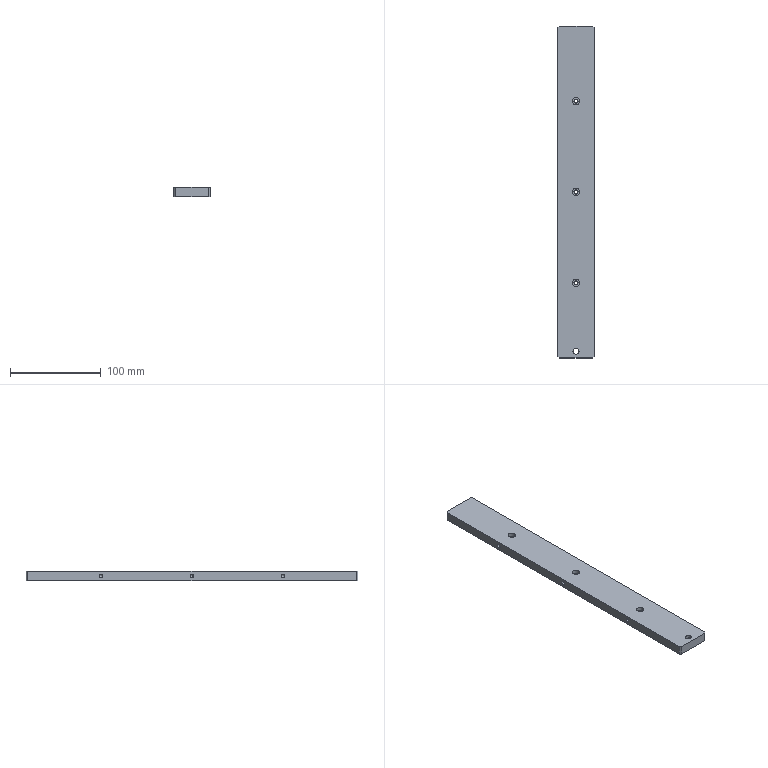Part | SolidWorks | features MirrorStock 1 | 1 solid | 50 faces | box 40 x 365 x 10 mm | volume 143435 mm3 | cylinder 26 | plane 14 | cone 10 | commonest cylinder face diameters 4.2 x6 4.5 x6 8 x6 3.3 x4 6.6 x2 11 x2
STEP:
#1=CARTESIAN_POINT('',(-4.,100.,0.4));
#2=VERTEX_POINT('',#1);
#3=CARTESIAN_POINT('',(4.,100.,0.4));
#4=VERTEX_POINT('',#3);
#5=CARTESIAN_POINT('',(0.,100.,0.4));
#6=DIRECTION('',(0.,0.,-1.));
#7=DIRECTION('',(-1.,0.,0.));
#8=AXIS2_PLACEMENT_3D('',#5,#6,#7);
#9=CIRCLE('',#8,4.);
#10=EDGE_CURVE('',#2,#4,#9,.T.);
#11=ORIENTED_EDGE('',*,*,#10,.T.);
#12=CARTESIAN_POINT('',(4.,100.,5.));
#13=VERTEX_POINT('',#12);
#14=CARTESIAN_POINT('',(4.,100.,5.));
#15=DIRECTION('',(0.,0.,1.));
#16=VECTOR('',#15,1000.);
#17=LINE('',#14,#16);
#18=EDGE_CURVE('',#4,#13,#17,.T.);
#19=ORIENTED_EDGE('',*,*,#18,.T.);
#20=CARTESIAN_POINT('',(-4.,100.,5.));
#21=VERTEX_POINT('',#20);
#22=CARTESIAN_POINT('',(0.,100.,5.));
#23=DIRECTION('',(0.,0.,-1.));
#24=DIRECTION('',(-1.,0.,0.));
#25=AXIS2_PLACEMENT_3D('',#22,#23,#24);
#26=CIRCLE('',#25,4.);
#27=EDGE_CURVE('',#21,#13,#26,.T.);
#28=ORIENTED_EDGE('',*,*,#27,.F.);
#29=CARTESIAN_POINT('',(-4.,100.,5.));
#30=DIRECTION('',(0.,0.,1.));
#31=VECTOR('',#30,1000.);
#32=LINE('',#29,#31);
#33=EDGE_CURVE('',#2,#21,#32,.T.);
#34=ORIENTED_EDGE('',*,*,#33,.F.);
#35=EDGE_LOOP('',(#11,#19,#28,#34));
#36=FACE_OUTER_BOUND('',#35,.T.);
#37=CARTESIAN_POINT('',(0.,100.,5.));
#38=DIRECTION('',(0.,0.,1.));
#39=DIRECTION('',(-1.,0.,0.));
#40=AXIS2_PLACEMENT_3D('',#37,#38,#39);
#41=CYLINDRICAL_SURFACE('',#40,4.);
#42=ADVANCED_FACE('',(#36),#41,.F.);
#43=CARTESIAN_POINT('',(-2.25,100.,-5.));
#44=VERTEX_POINT('',#43);
#45=CARTESIAN_POINT('',(2.25,100.,-5.));
#46=VERTEX_POINT('',#45);
#47=CARTESIAN_POINT('',(0.,100.,-5.));
#48=DIRECTION('',(0.,0.,-1.));
#49=DIRECTION('',(-1.,0.,0.));
#50=AXIS2_PLACEMENT_3D('',#47,#48,#49);
#51=CIRCLE('',#50,2.25);
#52=EDGE_CURVE('',#44,#46,#51,.T.);
#53=ORIENTED_EDGE('',*,*,#52,.T.);
#54=CARTESIAN_POINT('',(2.25,100.,0.4));
#55=VERTEX_POINT('',#54);
#56=CARTESIAN_POINT('',(2.25,100.,5.));
#57=DIRECTION('',(0.,0.,1.));
#58=VECTOR('',#57,1000.);
#59=LINE('',#56,#58);
#60=EDGE_CURVE('',#46,#55,#59,.T.);
#61=ORIENTED_EDGE('',*,*,#60,.T.);
#62=CARTESIAN_POINT('',(-2.25,100.,0.4));
#63=VERTEX_POINT('',#62);
#64=CARTESIAN_POINT('',(0.,100.,0.4));
#65=DIRECTION('',(0.,0.,-1.));
#66=DIRECTION('',(-1.,0.,0.));
#67=AXIS2_PLACEMENT_3D('',#64,#65,#66);
#68=CIRCLE('',#67,2.25);
#69=EDGE_CURVE('',#63,#55,#68,.T.);
#70=ORIENTED_EDGE('',*,*,#69,.F.);
#71=CARTESIAN_POINT('',(-2.25,100.,5.));
#72=DIRECTION('',(0.,0.,1.));
#73=VECTOR('',#72,1000.);
#74=LINE('',#71,#73);
#75=EDGE_CURVE('',#44,#63,#74,.T.);
#76=ORIENTED_EDGE('',*,*,#75,.F.);
#77=EDGE_LOOP('',(#53,#61,#70,#76));
#78=FACE_OUTER_BOUND('',#77,.T.);
#79=CARTESIAN_POINT('',(0.,100.,5.));
#80=DIRECTION('',(0.,0.,1.));
#81=DIRECTION('',(-1.,0.,0.));
#82=AXIS2_PLACEMENT_3D('',#79,#80,#81);
#83=CYLINDRICAL_SURFACE('',#82,2.25);
#84=ADVANCED_FACE('',(#78),#83,.F.);
#85=CARTESIAN_POINT('',(-4.,0.,0.4));
#86=VERTEX_POINT('',#85);
#87=CARTESIAN_POINT('',(4.,0.,0.4));
#88=VERTEX_POINT('',#87);
#89=CARTESIAN_POINT('',(0.,0.,0.4));
#90=DIRECTION('',(0.,0.,-1.));
#91=DIRECTION('',(-1.,0.,0.));
#92=AXIS2_PLACEMENT_3D('',#89,#90,#91);
#93=CIRCLE('',#92,4.);
#94=EDGE_CURVE('',#86,#88,#93,.T.);
#95=ORIENTED_EDGE('',*,*,#94,.T.);
#96=CARTESIAN_POINT('',(4.,0.,5.));
#97=VERTEX_POINT('',#96);
#98=CARTESIAN_POINT('',(4.,0.,5.));
#99=DIRECTION('',(0.,0.,1.));
#100=VECTOR('',#99,1000.);
#101=LINE('',#98,#100);
#102=EDGE_CURVE('',#88,#97,#101,.T.);
#103=ORIENTED_EDGE('',*,*,#102,.T.);
#104=CARTESIAN_POINT('',(-4.,0.,5.));
#105=VERTEX_POINT('',#104);
#106=CARTESIAN_POINT('',(0.,0.,5.));
#107=DIRECTION('',(0.,0.,-1.));
#108=DIRECTION('',(-1.,0.,0.));
#109=AXIS2_PLACEMENT_3D('',#106,#107,#108);
#110=CIRCLE('',#109,4.);
#111=EDGE_CURVE('',#105,#97,#110,.T.);
#112=ORIENTED_EDGE('',*,*,#111,.F.);
#113=CARTESIAN_POINT('',(-4.,0.,5.));
#114=DIRECTION('',(0.,0.,1.));
#115=VECTOR('',#114,1000.);
#116=LINE('',#113,#115);
#117=EDGE_CURVE('',#86,#105,#116,.T.);
#118=ORIENTED_EDGE('',*,*,#117,.F.);
#119=EDGE_LOOP('',(#95,#103,#112,#118));
#120=FACE_OUTER_BOUND('',#119,.T.);
#121=CARTESIAN_POINT('',(0.,0.,5.));
#122=DIRECTION('',(0.,0.,1.));
#123=DIRECTION('',(-1.,0.,0.));
#124=AXIS2_PLACEMENT_3D('',#121,#122,#123);
#125=CYLINDRICAL_SURFACE('',#124,4.);
#126=ADVANCED_FACE('',(#120),#125,.F.);
#127=CARTESIAN_POINT('',(-2.25,0.,-5.));
#128=VERTEX_POINT('',#127);
#129=CARTESIAN_POINT('',(2.25,0.,-5.));
#130=VERTEX_POINT('',#129);
#131=CARTESIAN_POINT('',(0.,0.,-5.));
#132=DIRECTION('',(0.,0.,-1.));
#133=DIRECTION('',(-1.,0.,0.));
#134=AXIS2_PLACEMENT_3D('',#131,#132,#133);
#135=CIRCLE('',#134,2.25);
#136=EDGE_CURVE('',#128,#130,#135,.T.);
#137=ORIENTED_EDGE('',*,*,#136,.T.);
#138=CARTESIAN_POINT('',(2.25,0.,0.4));
#139=VERTEX_POINT('',#138);
#140=CARTESIAN_POINT('',(2.25,0.,5.));
#141=DIRECTION('',(0.,0.,1.));
#142=VECTOR('',#141,1000.);
#143=LINE('',#140,#142);
#144=EDGE_CURVE('',#130,#139,#143,.T.);
#145=ORIENTED_EDGE('',*,*,#144,.T.);
#146=CARTESIAN_POINT('',(-2.25,0.,0.4));
#147=VERTEX_POINT('',#146);
#148=CARTESIAN_POINT('',(0.,0.,0.4));
#149=DIRECTION('',(0.,0.,-1.));
#150=DIRECTION('',(-1.,0.,0.));
#151=AXIS2_PLACEMENT_3D('',#148,#149,#150);
#152=CIRCLE('',#151,2.25);
#153=EDGE_CURVE('',#147,#139,#152,.T.);
#154=ORIENTED_EDGE('',*,*,#153,.F.);
#155=CARTESIAN_POINT('',(-2.25,0.,5.));
#156=DIRECTION('',(0.,0.,1.));
#157=VECTOR('',#156,1000.);
#158=LINE('',#155,#157);
#159=EDGE_CURVE('',#128,#147,#158,.T.);
#160=ORIENTED_EDGE('',*,*,#159,.F.);
#161=EDGE_LOOP('',(#137,#145,#154,#160));
#162=FACE_OUTER_BOUND('',#161,.T.);
#163=CARTESIAN_POINT('',(0.,0.,5.));
#164=DIRECTION('',(0.,0.,1.));
#165=DIRECTION('',(-1.,0.,0.));
#166=AXIS2_PLACEMENT_3D('',#163,#164,#165);
#167=CYLINDRICAL_SURFACE('',#166,2.25);
#168=ADVANCED_FACE('',(#162),#167,.F.);
#169=CARTESIAN_POINT('',(-4.,-100.,0.4));
#170=VERTEX_POINT('',#169);
#171=CARTESIAN_POINT('',(4.,-100.,0.4));
#172=VERTEX_POINT('',#171);
#173=CARTESIAN_POINT('',(0.,-100.,0.4));
#174=DIRECTION('',(0.,0.,-1.));
#175=DIRECTION('',(-1.,0.,0.));
#176=AXIS2_PLACEMENT_3D('',#173,#174,#175);
#177=CIRCLE('',#176,4.);
#178=EDGE_CURVE('',#170,#172,#177,.T.);
#179=ORIENTED_EDGE('',*,*,#178,.T.);
#180=CARTESIAN_POINT('',(4.,-100.,5.));
#181=VERTEX_POINT('',#180);
#182=CARTESIAN_POINT('',(4.,-100.,5.));
#183=DIRECTION('',(0.,0.,1.));
#184=VECTOR('',#183,1000.);
#185=LINE('',#182,#184);
#186=EDGE_CURVE('',#172,#181,#185,.T.);
#187=ORIENTED_EDGE('',*,*,#186,.T.);
#188=CARTESIAN_POINT('',(-4.,-100.,5.));
#189=VERTEX_POINT('',#188);
#190=CARTESIAN_POINT('',(0.,-100.,5.));
#191=DIRECTION('',(0.,0.,-1.));
#192=DIRECTION('',(-1.,0.,0.));
#193=AXIS2_PLACEMENT_3D('',#190,#191,#192);
#194=CIRCLE('',#193,4.);
#195=EDGE_CURVE('',#189,#181,#194,.T.);
#196=ORIENTED_EDGE('',*,*,#195,.F.);
#197=CARTESIAN_POINT('',(-4.,-100.,5.));
#198=DIRECTION('',(0.,0.,1.));
#199=VECTOR('',#198,1000.);
#200=LINE('',#197,#199);
#201=EDGE_CURVE('',#170,#189,#200,.T.);
#202=ORIENTED_EDGE('',*,*,#201,.F.);
#203=EDGE_LOOP('',(#179,#187,#196,#202));
#204=FACE_OUTER_BOUND('',#203,.T.);
#205=CARTESIAN_POINT('',(0.,-100.,5.));
#206=DIRECTION('',(0.,0.,1.));
#207=DIRECTION('',(-1.,0.,0.));
#208=AXIS2_PLACEMENT_3D('',#205,#206,#207);
#209=CYLINDRICAL_SURFACE('',#208,4.);
#210=ADVANCED_FACE('',(#204),#209,.F.);
#211=CARTESIAN_POINT('',(-2.25,-100.,-5.));
#212=VERTEX_POINT('',#211);
#213=CARTESIAN_POINT('',(2.25,-100.,-5.));
#214=VERTEX_POINT('',#213);
#215=CARTESIAN_POINT('',(0.,-100.,-5.));
#216=DIRECTION('',(0.,0.,-1.));
#217=DIRECTION('',(-1.,0.,0.));
#218=AXIS2_PLACEMENT_3D('',#215,#216,#217);
#219=CIRCLE('',#218,2.25);
#220=EDGE_CURVE('',#212,#214,#219,.T.);
#221=ORIENTED_EDGE('',*,*,#220,.T.);
#222=CARTESIAN_POINT('',(2.25,-100.,0.4));
#223=VERTEX_POINT('',#222);
#224=CARTESIAN_POINT('',(2.25,-100.,5.));
#225=DIRECTION('',(0.,0.,1.));
#226=VECTOR('',#225,1000.);
#227=LINE('',#224,#226);
#228=EDGE_CURVE('',#214,#223,#227,.T.);
#229=ORIENTED_EDGE('',*,*,#228,.T.);
#230=CARTESIAN_POINT('',(-2.25,-100.,0.4));
#231=VERTEX_POINT('',#230);
#232=CARTESIAN_POINT('',(0.,-100.,0.4));
#233=DIRECTION('',(0.,0.,-1.));
#234=DIRECTION('',(-1.,0.,0.));
#235=AXIS2_PLACEMENT_3D('',#232,#233,#234);
#236=CIRCLE('',#235,2.25);
#237=EDGE_CURVE('',#231,#223,#236,.T.);
#238=ORIENTED_EDGE('',*,*,#237,.F.);
#239=CARTESIAN_POINT('',(-2.25,-100.,5.));
#240=DIRECTION('',(0.,0.,1.));
#241=VECTOR('',#240,1000.);
#242=LINE('',#239,#241);
#243=EDGE_CURVE('',#212,#231,#242,.T.);
#244=ORIENTED_EDGE('',*,*,#243,.F.);
#245=EDGE_LOOP('',(#221,#229,#238,#244));
#246=FACE_OUTER_BOUND('',#245,.T.);
#247=CARTESIAN_POINT('',(0.,-100.,5.));
#248=DIRECTION('',(0.,0.,1.));
#249=DIRECTION('',(-1.,0.,0.));
#250=AXIS2_PLACEMENT_3D('',#247,#248,#249);
#251=CYLINDRICAL_SURFACE('',#250,2.25);
#252=ADVANCED_FACE('',(#246),#251,.F.);
#253=CARTESIAN_POINT('',(-6.,0.,-2.1));
#254=VERTEX_POINT('',#253);
#255=CARTESIAN_POINT('',(-6.,0.,2.1));
#256=VERTEX_POINT('',#255);
#257=CARTESIAN_POINT('',(-6.,0.,0.));
#258=DIRECTION('',(1.,0.,0.));
#259=DIRECTION('',(0.,0.,-1.));
#260=AXIS2_PLACEMENT_3D('',#257,#258,#259);
#261=CIRCLE('',#260,2.1);
#262=EDGE_CURVE('',#254,#256,#261,.T.);
#263=ORIENTED_EDGE('',*,*,#262,.T.);
#264=CARTESIAN_POINT('',(-20.,0.,2.1));
#265=VERTEX_POINT('',#264);
#266=CARTESIAN_POINT('',(-20.,0.,2.1));
#267=DIRECTION('',(-1.,0.,0.));
#268=VECTOR('',#267,1000.);
#269=LINE('',#266,#268);
#270=EDGE_CURVE('',#256,#265,#269,.T.);
#271=ORIENTED_EDGE('',*,*,#270,.T.);
#272=CARTESIAN_POINT('',(-20.,0.,-2.1));
#273=VERTEX_POINT('',#272);
#274=CARTESIAN_POINT('',(-20.,0.,0.));
#275=DIRECTION('',(1.,0.,0.));
#276=DIRECTION('',(0.,0.,-1.));
#277=AXIS2_PLACEMENT_3D('',#274,#275,#276);
#278=CIRCLE('',#277,2.1);
#279=EDGE_CURVE('',#273,#265,#278,.T.);
#280=ORIENTED_EDGE('',*,*,#279,.F.);
#281=CARTESIAN_POINT('',(-20.,0.,-2.1));
#282=DIRECTION('',(-1.,0.,0.));
#283=VECTOR('',#282,1000.);
#284=LINE('',#281,#283);
#285=EDGE_CURVE('',#254,#273,#284,.T.);
#286=ORIENTED_EDGE('',*,*,#285,.F.);
#287=EDGE_LOOP('',(#263,#271,#280,#286));
#288=FACE_OUTER_BOUND('',#287,.T.);
#289=CARTESIAN_POINT('',(-20.,0.,0.));
#290=DIRECTION('',(-1.,0.,0.));
#291=DIRECTION('',(0.,0.,-1.));
#292=AXIS2_PLACEMENT_3D('',#289,#290,#291);
#293=CYLINDRICAL_SURFACE('',#292,2.1);
#294=ADVANCED_FACE('',(#288),#293,.F.);
#295=CARTESIAN_POINT('',(-4.738,0.,0.));
#296=VERTEX_POINT('',#295);
#297=CARTESIAN_POINT('',(-6.,0.,-2.1));
#298=DIRECTION('',(-0.515,0.,-0.8572));
#299=VECTOR('',#298,1000.);
#300=LINE('',#297,#299);
#301=EDGE_CURVE('',#296,#254,#300,.T.);
#302=ORIENTED_EDGE('',*,*,#301,.F.);
#303=CARTESIAN_POINT('',(-6.,0.,2.1));
#304=DIRECTION('',(-0.515,0.,0.8572));
#305=VECTOR('',#304,1000.);
#306=LINE('',#303,#305);
#307=EDGE_CURVE('',#296,#256,#306,.T.);
#308=ORIENTED_EDGE('',*,*,#307,.T.);
#309=ORIENTED_EDGE('',*,*,#262,.F.);
#310=EDGE_LOOP('',(#302,#308,#309));
#311=FACE_OUTER_BOUND('',#310,.T.);
#312=CARTESIAN_POINT('',(-6.,0.,0.));
#313=DIRECTION('',(-1.,0.,0.));
#314=DIRECTION('',(0.,0.,-1.));
#315=AXIS2_PLACEMENT_3D('',#312,#313,#314);
#316=CONICAL_SURFACE('',#315,2.1,1.03);
#317=ADVANCED_FACE('',(#311),#316,.F.);
#318=CARTESIAN_POINT('',(-6.,100.,-2.1));
#319=VERTEX_POINT('',#318);
#320=CARTESIAN_POINT('',(-6.,100.,2.1));
#321=VERTEX_POINT('',#320);
#322=CARTESIAN_POINT('',(-6.,100.,0.));
#323=DIRECTION('',(1.,0.,0.));
#324=DIRECTION('',(0.,0.,-1.));
#325=AXIS2_PLACEMENT_3D('',#322,#323,#324);
#326=CIRCLE('',#325,2.1);
#327=EDGE_CURVE('',#319,#321,#326,.T.);
#328=ORIENTED_EDGE('',*,*,#327,.T.);
#329=CARTESIAN_POINT('',(-20.,100.,2.1));
#330=VERTEX_POINT('',#329);
#331=CARTESIAN_POINT('',(-20.,100.,2.1));
#332=DIRECTION('',(-1.,0.,0.));
#333=VECTOR('',#332,1000.);
#334=LINE('',#331,#333);
#335=EDGE_CURVE('',#321,#330,#334,.T.);
#336=ORIENTED_EDGE('',*,*,#335,.T.);
#337=CARTESIAN_POINT('',(-20.,100.,-2.1));
#338=VERTEX_POINT('',#337);
#339=CARTESIAN_POINT('',(-20.,100.,0.));
#340=DIRECTION('',(1.,0.,0.));
#341=DIRECTION('',(0.,0.,-1.));
#342=AXIS2_PLACEMENT_3D('',#339,#340,#341);
#343=CIRCLE('',#342,2.1);
#344=EDGE_CURVE('',#338,#330,#343,.T.);
#345=ORIENTED_EDGE('',*,*,#344,.F.);
#346=CARTESIAN_POINT('',(-20.,100.,-2.1));
#347=DIRECTION('',(-1.,0.,0.));
#348=VECTOR('',#347,1000.);
#349=LINE('',#346,#348);
#350=EDGE_CURVE('',#319,#338,#349,.T.);
#351=ORIENTED_EDGE('',*,*,#350,.F.);
#352=EDGE_LOOP('',(#328,#336,#345,#351));
#353=FACE_OUTER_BOUND('',#352,.T.);
#354=CARTESIAN_POINT('',(-20.,100.,0.));
#355=DIRECTION('',(-1.,0.,0.));
#356=DIRECTION('',(0.,0.,-1.));
#357=AXIS2_PLACEMENT_3D('',#354,#355,#356);
#358=CYLINDRICAL_SURFACE('',#357,2.1);
#359=ADVANCED_FACE('',(#353),#358,.F.);
#360=CARTESIAN_POINT('',(-4.738,100.,0.));
#361=VERTEX_POINT('',#360);
#362=CARTESIAN_POINT('',(-6.,100.,-2.1));
#363=DIRECTION('',(-0.515,0.,-0.8572));
#364=VECTOR('',#363,1000.);
#365=LINE('',#362,#364);
#366=EDGE_CURVE('',#361,#319,#365,.T.);
#367=ORIENTED_EDGE('',*,*,#366,.F.);
#368=CARTESIAN_POINT('',(-6.,100.,2.1));
#369=DIRECTION('',(-0.515,0.,0.8572));
#370=VECTOR('',#369,1000.);
#371=LINE('',#368,#370);
#372=EDGE_CURVE('',#361,#321,#371,.T.);
#373=ORIENTED_EDGE('',*,*,#372,.T.);
#374=ORIENTED_EDGE('',*,*,#327,.F.);
#375=EDGE_LOOP('',(#367,#373,#374));
#376=FACE_OUTER_BOUND('',#375,.T.);
#377=CARTESIAN_POINT('',(-6.,100.,0.));
#378=DIRECTION('',(-1.,0.,0.));
#379=DIRECTION('',(0.,0.,-1.));
#380=AXIS2_PLACEMENT_3D('',#377,#378,#379);
#381=CONICAL_SURFACE('',#380,2.1,1.03);
#382=ADVANCED_FACE('',(#376),#381,.F.);
#383=CARTESIAN_POINT('',(-6.,-100.,-2.1));
#384=VERTEX_POINT('',#383);
#385=CARTESIAN_POINT('',(-6.,-100.,2.1));
#386=VERTEX_POINT('',#385);
#387=CARTESIAN_POINT('',(-6.,-100.,0.));
#388=DIRECTION('',(1.,0.,0.));
#389=DIRECTION('',(0.,0.,-1.));
#390=AXIS2_PLACEMENT_3D('',#387,#388,#389);
#391=CIRCLE('',#390,2.1);
#392=EDGE_CURVE('',#384,#386,#391,.T.);
#393=ORIENTED_EDGE('',*,*,#392,.T.);
#394=CARTESIAN_POINT('',(-20.,-100.,2.1));
#395=VERTEX_POINT('',#394);
#396=CARTESIAN_POINT('',(-20.,-100.,2.1));
#397=DIRECTION('',(-1.,0.,0.));
#398=VECTOR('',#397,1000.);
#399=LINE('',#396,#398);
#400=EDGE_CURVE('',#386,#395,#399,.T.);
#401=ORIENTED_EDGE('',*,*,#400,.T.);
#402=CARTESIAN_POINT('',(-20.,-100.,-2.1));
#403=VERTEX_POINT('',#402);
#404=CARTESIAN_POINT('',(-20.,-100.,0.));
#405=DIRECTION('',(1.,0.,0.));
#406=DIRECTION('',(0.,0.,-1.));
#407=AXIS2_PLACEMENT_3D('',#404,#405,#406);
#408=CIRCLE('',#407,2.1);
#409=EDGE_CURVE('',#403,#395,#408,.T.);
#410=ORIENTED_EDGE('',*,*,#409,.F.);
#411=CARTESIAN_POINT('',(-20.,-100.,-2.1));
#412=DIRECTION('',(-1.,0.,0.));
#413=VECTOR('',#412,1000.);
#414=LINE('',#411,#413);
#415=EDGE_CURVE('',#384,#403,#414,.T.);
#416=ORIENTED_EDGE('',*,*,#415,.F.);
#417=EDGE_LOOP('',(#393,#401,#410,#416));
#418=FACE_OUTER_BOUND('',#417,.T.);
#419=CARTESIAN_POINT('',(-20.,-100.,0.));
#420=DIRECTION('',(-1.,0.,0.));
#421=DIRECTION('',(0.,0.,-1.));
#422=AXIS2_PLACEMENT_3D('',#419,#420,#421);
#423=CYLINDRICAL_SURFACE('',#422,2.1);
#424=ADVANCED_FACE('',(#418),#423,.F.);
#425=CARTESIAN_POINT('',(-4.738,-100.,0.));
#426=VERTEX_POINT('',#425);
#427=CARTESIAN_POINT('',(-6.,-100.,-2.1));
#428=DIRECTION('',(-0.515,0.,-0.8572));
#429=VECTOR('',#428,1000.);
#430=LINE('',#427,#429);
#431=EDGE_CURVE('',#426,#384,#430,.T.);
#432=ORIENTED_EDGE('',*,*,#431,.F.);
#433=CARTESIAN_POINT('',(-6.,-100.,2.1));
#434=DIRECTION('',(-0.515,0.,0.8572));
#435=VECTOR('',#434,1000.);
#436=LINE('',#433,#435);
#437=EDGE_CURVE('',#426,#386,#436,.T.);
#438=ORIENTED_EDGE('',*,*,#437,.T.);
#439=ORIENTED_EDGE('',*,*,#392,.F.);
#440=EDGE_LOOP('',(#432,#438,#439));
#441=FACE_OUTER_BOUND('',#440,.T.);
#442=CARTESIAN_POINT('',(-6.,-100.,0.));
#443=DIRECTION('',(-1.,0.,0.));
#444=DIRECTION('',(0.,0.,-1.));
#445=AXIS2_PLACEMENT_3D('',#442,#443,#444);
#446=CONICAL_SURFACE('',#445,2.1,1.03);
#447=ADVANCED_FACE('',(#441),#446,.F.);
#448=CARTESIAN_POINT('',(5.5,-175.,1.8));
#449=VERTEX_POINT('',#448);
#450=CARTESIAN_POINT('',(-5.5,-175.,1.8));
#451=VERTEX_POINT('',#450);
#452=CARTESIAN_POINT('',(0.,-175.,1.8));
#453=DIRECTION('',(0.,0.,1.));
#454=DIRECTION('',(1.,0.,0.));
#455=AXIS2_PLACEMENT_3D('',#452,#453,#454);
#456=CIRCLE('',#455,5.5);
#457=EDGE_CURVE('',#449,#451,#456,.T.);
#458=ORIENTED_EDGE('',*,*,#457,.T.);
#459=CARTESIAN_POINT('',(-5.5,-175.,-5.));
#460=VERTEX_POINT('',#459);
#461=CARTESIAN_POINT('',(-5.5,-175.,-5.));
#462=DIRECTION('',(0.,0.,-1.));
#463=VECTOR('',#462,1000.);
#464=LINE('',#461,#463);
#465=EDGE_CURVE('',#451,#460,#464,.T.);
#466=ORIENTED_EDGE('',*,*,#465,.T.);
#467=CARTESIAN_POINT('',(5.5,-175.,-5.));
#468=VERTEX_POINT('',#467);
#469=CARTESIAN_POINT('',(0.,-175.,-5.));
#470=DIRECTION('',(0.,0.,1.));
#471=DIRECTION('',(1.,0.,0.));
#472=AXIS2_PLACEMENT_3D('',#469,#470,#471);
#473=CIRCLE('',#472,5.5);
#474=EDGE_CURVE('',#468,#460,#473,.T.);
#475=ORIENTED_EDGE('',*,*,#474,.F.);
#476=CARTESIAN_POINT('',(5.5,-175.,-5.));
#477=DIRECTION('',(0.,0.,-1.));
#478=VECTOR('',#477,1000.);
#479=LINE('',#476,#478);
#480=EDGE_CURVE('',#449,#468,#479,.T.);
#481=ORIENTED_EDGE('',*,*,#480,.F.);
#482=EDGE_LOOP('',(#458,#466,#475,#481));
#483=FACE_OUTER_BOUND('',#482,.T.);
#484=CARTESIAN_POINT('',(0.,-175.,-5.));
#485=DIRECTION('',(0.,0.,-1.));
#486=DIRECTION('',(1.,0.,0.));
#487=AXIS2_PLACEMENT_3D('',#484,#485,#486);
#488=CYLINDRICAL_SURFACE('',#487,5.5);
#489=ADVANCED_FACE('',(#483),#488,.F.);
#490=CARTESIAN_POINT('',(3.3,-175.,5.));
#491=VERTEX_POINT('',#490);
#492=CARTESIAN_POINT('',(-3.3,-175.,5.));
#493=VERTEX_POINT('',#492);
#494=CARTESIAN_POINT('',(0.,-175.,5.));
#495=DIRECTION('',(0.,0.,1.));
#496=DIRECTION('',(1.,0.,0.));
#497=AXIS2_PLACEMENT_3D('',#494,#495,#496);
#498=CIRCLE('',#497,3.3);
#499=EDGE_CURVE('',#491,#493,#498,.T.);
#500=ORIENTED_EDGE('',*,*,#499,.T.);
#501=CARTESIAN_POINT('',(-3.3,-175.,1.8));
#502=VERTEX_POINT('',#501);
#503=CARTESIAN_POINT('',(-3.3,-175.,-5.));
#504=DIRECTION('',(0.,0.,-1.));
#505=VECTOR('',#504,1000.);
#506=LINE('',#503,#505);
#507=EDGE_CURVE('',#493,#502,#506,.T.);
#508=ORIENTED_EDGE('',*,*,#507,.T.);
#509=CARTESIAN_POINT('',(3.3,-175.,1.8));
#510=VERTEX_POINT('',#509);
#511=CARTESIAN_POINT('',(0.,-175.,1.8));
#512=DIRECTION('',(0.,0.,1.));
#513=DIRECTION('',(1.,0.,0.));
#514=AXIS2_PLACEMENT_3D('',#511,#512,#513);
#515=CIRCLE('',#514,3.3);
#516=EDGE_CURVE('',#510,#502,#515,.T.);
#517=ORIENTED_EDGE('',*,*,#516,.F.);
#518=CARTESIAN_POINT('',(3.3,-175.,-5.));
#519=DIRECTION('',(0.,0.,-1.));
#520=VECTOR('',#519,1000.);
#521=LINE('',#518,#520);
#522=EDGE_CURVE('',#491,#510,#521,.T.);
#523=ORIENTED_EDGE('',*,*,#522,.F.);
#524=EDGE_LOOP('',(#500,#508,#517,#523));
#525=FACE_OUTER_BOUND('',#524,.T.);
#526=CARTESIAN_POINT('',(0.,-175.,-5.));
#527=DIRECTION('',(0.,0.,-1.));
#528=DIRECTION('',(1.,0.,0.));
#529=AXIS2_PLACEMENT_3D('',#526,#527,#528);
#530=CYLINDRICAL_SURFACE('',#529,3.3);
#531=ADVANCED_FACE('',(#525),#530,.F.);
#532=CARTESIAN_POINT('',(-10.,172.4,-1.65));
#533=VERTEX_POINT('',#532);
#534=CARTESIAN_POINT('',(-10.,172.4,1.65));
#535=VERTEX_POINT('',#534);
#536=CARTESIAN_POINT('',(-10.,172.4,0.));
#537=DIRECTION('',(0.,-1.,0.));
#538=DIRECTION('',(0.,0.,-1.));
#539=AXIS2_PLACEMENT_3D('',#536,#537,#538);
#540=CIRCLE('',#539,1.65);
#541=EDGE_CURVE('',#533,#535,#540,.T.);
#542=ORIENTED_EDGE('',*,*,#541,.T.);
#543=CARTESIAN_POINT('',(-10.,182.5,1.65));
#544=VERTEX_POINT('',#543);
#545=CARTESIAN_POINT('',(-10.,182.5,1.65));
#546=DIRECTION('',(0.,1.,0.));
#547=VECTOR('',#546,1000.);
#548=LINE('',#545,#547);
#549=EDGE_CURVE('',#535,#544,#548,.T.);
#550=ORIENTED_EDGE('',*,*,#549,.T.);
#551=CARTESIAN_POINT('',(-10.,182.5,-1.65));
#552=VERTEX_POINT('',#551);
#553=CARTESIAN_POINT('',(-10.,182.5,0.));
#554=DIRECTION('',(0.,-1.,0.));
#555=DIRECTION('',(0.,0.,-1.));
#556=AXIS2_PLACEMENT_3D('',#553,#554,#555);
#557=CIRCLE('',#556,1.65);
#558=EDGE_CURVE('',#552,#544,#557,.T.);
#559=ORIENTED_EDGE('',*,*,#558,.F.);
#560=CARTESIAN_POINT('',(-10.,182.5,-1.65));
#561=DIRECTION('',(0.,1.,0.));
#562=VECTOR('',#561,1000.);
#563=LINE('',#560,#562);
#564=EDGE_CURVE('',#533,#552,#563,.T.);
#565=ORIENTED_EDGE('',*,*,#564,.F.);
#566=EDGE_LOOP('',(#542,#550,#559,#565));
#567=FACE_OUTER_BOUND('',#566,.T.);
#568=CARTESIAN_POINT('',(-10.,182.5,0.));
#569=DIRECTION('',(0.,1.,0.));
#570=DIRECTION('',(0.,0.,-1.));
#571=AXIS2_PLACEMENT_3D('',#568,#569,#570);
#572=CYLINDRICAL_SURFACE('',#571,1.65);
#573=ADVANCED_FACE('',(#567),#572,.F.);
#574=CARTESIAN_POINT('',(-10.,171.409,0.));
#575=VERTEX_POINT('',#574);
#576=CARTESIAN_POINT('',(-10.,172.4,-1.65));
#577=DIRECTION('',(0.,0.515,-0.8572));
#578=VECTOR('',#577,1000.);
#579=LINE('',#576,#578);
#580=EDGE_CURVE('',#575,#533,#579,.T.);
#581=ORIENTED_EDGE('',*,*,#580,.F.);
#582=CARTESIAN_POINT('',(-10.,172.4,1.65));
#583=DIRECTION('',(0.,0.515,0.8572));
#584=VECTOR('',#583,1000.);
#585=LINE('',#582,#584);
#586=EDGE_CURVE('',#575,#535,#585,.T.);
#587=ORIENTED_EDGE('',*,*,#586,.T.);
#588=ORIENTED_EDGE('',*,*,#541,.F.);
#589=EDGE_LOOP('',(#581,#587,#588));
#590=FACE_OUTER_BOUND('',#589,.T.);
#591=CARTESIAN_POINT('',(-10.,172.4,0.));
#592=DIRECTION('',(0.,1.,0.));
#593=DIRECTION('',(0.,0.,-1.));
#594=AXIS2_PLACEMENT_3D('',#591,#592,#593);
#595=CONICAL_SURFACE('',#594,1.65,1.03);
#596=ADVANCED_FACE('',(#590),#595,.F.);
#597=CARTESIAN_POINT('',(10.,172.4,-1.65));
#598=VERTEX_POINT('',#597);
#599=CARTESIAN_POINT('',(10.,172.4,1.65));
#600=VERTEX_POINT('',#599);
#601=CARTESIAN_POINT('',(10.,172.4,0.));
#602=DIRECTION('',(0.,-1.,0.));
#603=DIRECTION('',(0.,0.,-1.));
#604=AXIS2_PLACEMENT_3D('',#601,#602,#603);
#605=CIRCLE('',#604,1.65);
#606=EDGE_CURVE('',#598,#600,#605,.T.);
#607=ORIENTED_EDGE('',*,*,#606,.T.);
#608=CARTESIAN_POINT('',(10.,182.5,1.65));
#609=VERTEX_POINT('',#608);
#610=CARTESIAN_POINT('',(10.,182.5,1.65));
#611=DIRECTION('',(0.,1.,0.));
#612=VECTOR('',#611,1000.);
#613=LINE('',#610,#612);
#614=EDGE_CURVE('',#600,#609,#613,.T.);
#615=ORIENTED_EDGE('',*,*,#614,.T.);
#616=CARTESIAN_POINT('',(10.,182.5,-1.65));
#617=VERTEX_POINT('',#616);
#618=CARTESIAN_POINT('',(10.,182.5,0.));
#619=DIRECTION('',(0.,-1.,0.));
#620=DIRECTION('',(0.,0.,-1.));
#621=AXIS2_PLACEMENT_3D('',#618,#619,#620);
#622=CIRCLE('',#621,1.65);
#623=EDGE_CURVE('',#617,#609,#622,.T.);
#624=ORIENTED_EDGE('',*,*,#623,.F.);
#625=CARTESIAN_POINT('',(10.,182.5,-1.65));
#626=DIRECTION('',(0.,1.,0.));
#627=VECTOR('',#626,1000.);
#628=LINE('',#625,#627);
#629=EDGE_CURVE('',#598,#617,#628,.T.);
#630=ORIENTED_EDGE('',*,*,#629,.F.);
#631=EDGE_LOOP('',(#607,#615,#624,#630));
#632=FACE_OUTER_BOUND('',#631,.T.);
#633=CARTESIAN_POINT('',(10.,182.5,0.));
#634=DIRECTION('',(0.,1.,0.));
#635=DIRECTION('',(0.,0.,-1.));
#636=AXIS2_PLACEMENT_3D('',#633,#634,#635);
#637=CYLINDRICAL_SURFACE('',#636,1.65);
#638=ADVANCED_FACE('',(#632),#637,.F.);
#639=CARTESIAN_POINT('',(10.,171.409,0.));
#640=VERTEX_POINT('',#639);
#641=CARTESIAN_POINT('',(10.,172.4,-1.65));
#642=DIRECTION('',(0.,0.515,-0.8572));
#643=VECTOR('',#642,1000.);
#644=LINE('',#641,#643);
#645=EDGE_CURVE('',#640,#598,#644,.T.);
#646=ORIENTED_EDGE('',*,*,#645,.F.);
#647=CARTESIAN_POINT('',(10.,172.4,1.65));
#648=DIRECTION('',(0.,0.515,0.8572));
#649=VECTOR('',#648,1000.);
#650=LINE('',#647,#649);
#651=EDGE_CURVE('',#640,#600,#650,.T.);
#652=ORIENTED_EDGE('',*,*,#651,.T.);
#653=ORIENTED_EDGE('',*,*,#606,.F.);
#654=EDGE_LOOP('',(#646,#652,#653));
#655=FACE_OUTER_BOUND('',#654,.T.);
#656=CARTESIAN_POINT('',(10.,172.4,0.));
#657=DIRECTION('',(0.,1.,0.));
#658=DIRECTION('',(0.,0.,-1.));
#659=AXIS2_PLACEMENT_3D('',#656,#657,#658);
#660=CONICAL_SURFACE('',#659,1.65,1.03);
#661=ADVANCED_FACE('',(#655),#660,.F.);
#662=ORIENTED_EDGE('',*,*,#279,.T.);
#663=CARTESIAN_POINT('',(-20.,0.,0.));
#664=DIRECTION('',(1.,0.,0.));
#665=DIRECTION('',(0.,0.,-1.));
#666=AXIS2_PLACEMENT_3D('',#663,#664,#665);
#667=CIRCLE('',#666,2.1);
#668=EDGE_CURVE('',#265,#273,#667,.T.);
#669=ORIENTED_EDGE('',*,*,#668,.T.);
#670=EDGE_LOOP('',(#662,#669));
#671=FACE_BOUND('',#670,.T.);
#672=ORIENTED_EDGE('',*,*,#344,.T.);
#673=CARTESIAN_POINT('',(-20.,100.,0.));
#674=DIRECTION('',(1.,0.,0.));
#675=DIRECTION('',(0.,0.,-1.));
#676=AXIS2_PLACEMENT_3D('',#673,#674,#675);
#677=CIRCLE('',#676,2.1);
#678=EDGE_CURVE('',#330,#338,#677,.T.);
#679=ORIENTED_EDGE('',*,*,#678,.T.);
#680=EDGE_LOOP('',(#672,#679));
#681=FACE_BOUND('',#680,.T.);
#682=ORIENTED_EDGE('',*,*,#409,.T.);
#683=CARTESIAN_POINT('',(-20.,-100.,0.));
#684=DIRECTION('',(1.,0.,0.));
#685=DIRECTION('',(0.,0.,-1.));
#686=AXIS2_PLACEMENT_3D('',#683,#684,#685);
#687=CIRCLE('',#686,2.1);
#688=EDGE_CURVE('',#395,#403,#687,.T.);
#689=ORIENTED_EDGE('',*,*,#688,.T.);
#690=EDGE_LOOP('',(#682,#689));
#691=FACE_BOUND('',#690,.T.);
#692=CARTESIAN_POINT('',(-20.,180.5,5.));
#693=VERTEX_POINT('',#692);
#694=CARTESIAN_POINT('',(-20.,-180.5,5.));
#695=VERTEX_POINT('',#694);
#696=CARTESIAN_POINT('',(-20.,-182.5,5.));
#697=DIRECTION('',(0.,-1.,0.));
#698=VECTOR('',#697,1000.);
#699=LINE('',#696,#698);
#700=EDGE_CURVE('',#693,#695,#699,.T.);
#701=ORIENTED_EDGE('',*,*,#700,.F.);
#702=CARTESIAN_POINT('',(-20.,180.5,-5.));
#703=VERTEX_POINT('',#702);
#704=CARTESIAN_POINT('',(-20.,180.5,-5.));
#705=DIRECTION('',(0.,0.,1.));
#706=VECTOR('',#705,1000.);
#707=LINE('',#704,#706);
#708=EDGE_CURVE('',#703,#693,#707,.T.);
#709=ORIENTED_EDGE('',*,*,#708,.F.);
#710=CARTESIAN_POINT('',(-20.,-180.5,-5.));
#711=VERTEX_POINT('',#710);
#712=CARTESIAN_POINT('',(-20.,-182.5,-5.));
#713=DIRECTION('',(0.,-1.,0.));
#714=VECTOR('',#713,1000.);
#715=LINE('',#712,#714);
#716=EDGE_CURVE('',#703,#711,#715,.T.);
#717=ORIENTED_EDGE('',*,*,#716,.T.);
#718=CARTESIAN_POINT('',(-20.,-180.5,-5.));
#719=DIRECTION('',(0.,0.,-1.));
#720=VECTOR('',#719,1000.);
#721=LINE('',#718,#720);
#722=EDGE_CURVE('',#695,#711,#721,.T.);
#723=ORIENTED_EDGE('',*,*,#722,.F.);
#724=EDGE_LOOP('',(#701,#709,#717,#723));
#725=FACE_OUTER_BOUND('',#724,.T.);
#726=CARTESIAN_POINT('',(-20.,-182.5,-5.));
#727=DIRECTION('',(1.,0.,0.));
#728=DIRECTION('',(0.,0.,1.));
#729=AXIS2_PLACEMENT_3D('',#726,#727,#728);
#730=PLANE('',#729);
#731=ADVANCED_FACE('',(#671,#681,#691,#725),#730,.F.);
#732=CARTESIAN_POINT('',(-18.,-182.5,-5.));
#733=VERTEX_POINT('',#732);
#734=CARTESIAN_POINT('',(18.,-182.5,-5.));
#735=VERTEX_POINT('',#734);
#736=CARTESIAN_POINT('',(20.,-182.5,-5.));
#737=DIRECTION('',(1.,0.,0.));
#738=VECTOR('',#737,1000.);
#739=LINE('',#736,#738);
#740=EDGE_CURVE('',#733,#735,#739,.T.);
#741=ORIENTED_EDGE('',*,*,#740,.T.);
#742=CARTESIAN_POINT('',(18.,-182.5,5.));
#743=VERTEX_POINT('',#742);
#744=CARTESIAN_POINT('',(18.,-182.5,-5.));
#745=DIRECTION('',(0.,0.,-1.));
#746=VECTOR('',#745,1000.);
#747=LINE('',#744,#746);
#748=EDGE_CURVE('',#743,#735,#747,.T.);
#749=ORIENTED_EDGE('',*,*,#748,.F.);
#750=CARTESIAN_POINT('',(-18.,-182.5,5.));
#751=VERTEX_POINT('',#750);
#752=CARTESIAN_POINT('',(20.,-182.5,5.));
#753=DIRECTION('',(1.,0.,0.));
#754=VECTOR('',#753,1000.);
#755=LINE('',#752,#754);
#756=EDGE_CURVE('',#751,#743,#755,.T.);
#757=ORIENTED_EDGE('',*,*,#756,.F.);
#758=CARTESIAN_POINT('',(-18.,-182.5,-5.));
#759=DIRECTION('',(0.,0.,1.));
#760=VECTOR('',#759,1000.);
#761=LINE('',#758,#760);
#762=EDGE_CURVE('',#733,#751,#761,.T.);
#763=ORIENTED_EDGE('',*,*,#762,.F.);
#764=EDGE_LOOP('',(#741,#749,#757,#763));
#765=FACE_OUTER_BOUND('',#764,.T.);
#766=CARTESIAN_POINT('',(20.,-182.5,-5.));
#767=DIRECTION('',(0.,1.,0.));
#768=DIRECTION('',(0.,0.,-1.));
#769=AXIS2_PLACEMENT_3D('',#766,#767,#768);
#770=PLANE('',#769);
#771=ADVANCED_FACE('',(#765),#770,.F.);
#772=CARTESIAN_POINT('',(20.,-180.5,-5.));
#773=VERTEX_POINT('',#772);
#774=CARTESIAN_POINT('',(20.,180.5,-5.));
#775=VERTEX_POINT('',#774);
#776=CARTESIAN_POINT('',(20.,-182.5,-5.));
#777=DIRECTION('',(0.,1.,0.));
#778=VECTOR('',#777,1000.);
#779=LINE('',#776,#778);
#780=EDGE_CURVE('',#773,#775,#779,.T.);
#781=ORIENTED_EDGE('',*,*,#780,.T.);
#782=CARTESIAN_POINT('',(20.,180.5,5.));
#783=VERTEX_POINT('',#782);
#784=CARTESIAN_POINT('',(20.,180.5,-5.));
#785=DIRECTION('',(0.,0.,-1.));
#786=VECTOR('',#785,1000.);
#787=LINE('',#784,#786);
#788=EDGE_CURVE('',#783,#775,#787,.T.);
#789=ORIENTED_EDGE('',*,*,#788,.F.);
#790=CARTESIAN_POINT('',(20.,-180.5,5.));
#791=VERTEX_POINT('',#790);
#792=CARTESIAN_POINT('',(20.,-182.5,5.));
#793=DIRECTION('',(0.,1.,0.));
#794=VECTOR('',#793,1000.);
#795=LINE('',#792,#794);
#796=EDGE_CURVE('',#791,#783,#795,.T.);
#797=ORIENTED_EDGE('',*,*,#796,.F.);
#798=CARTESIAN_POINT('',(20.,-180.5,-5.));
#799=DIRECTION('',(0.,0.,1.));
#800=VECTOR('',#799,1000.);
#801=LINE('',#798,#800);
#802=EDGE_CURVE('',#773,#791,#801,.T.);
#803=ORIENTED_EDGE('',*,*,#802,.F.);
#804=EDGE_LOOP('',(#781,#789,#797,#803));
#805=FACE_OUTER_BOUND('',#804,.T.);
#806=CARTESIAN_POINT('',(20.,-182.5,-5.));
#807=DIRECTION('',(-1.,0.,0.));
#808=DIRECTION('',(0.,0.,-1.));
#809=AXIS2_PLACEMENT_3D('',#806,#807,#808);
#810=PLANE('',#809);
#811=ADVANCED_FACE('',(#805),#810,.F.);
#812=ORIENTED_EDGE('',*,*,#558,.T.);
#813=CARTESIAN_POINT('',(-10.,182.5,0.));
#814=DIRECTION('',(0.,-1.,0.));
#815=DIRECTION('',(0.,0.,-1.));
#816=AXIS2_PLACEMENT_3D('',#813,#814,#815);
#817=CIRCLE('',#816,1.65);
#818=EDGE_CURVE('',#544,#552,#817,.T.);
#819=ORIENTED_EDGE('',*,*,#818,.T.);
#820=EDGE_LOOP('',(#812,#819));
#821=FACE_BOUND('',#820,.T.);
#822=ORIENTED_EDGE('',*,*,#623,.T.);
#823=CARTESIAN_POINT('',(10.,182.5,0.));
#824=DIRECTION('',(0.,-1.,0.));
#825=DIRECTION('',(0.,0.,-1.));
#826=AXIS2_PLACEMENT_3D('',#823,#824,#825);
#827=CIRCLE('',#826,1.65);
#828=EDGE_CURVE('',#609,#617,#827,.T.);
#829=ORIENTED_EDGE('',*,*,#828,.T.);
#830=EDGE_LOOP('',(#822,#829));
#831=FACE_BOUND('',#830,.T.);
#832=CARTESIAN_POINT('',(18.,182.5,5.));
#833=VERTEX_POINT('',#832);
#834=CARTESIAN_POINT('',(-18.,182.5,5.));
#835=VERTEX_POINT('',#834);
#836=CARTESIAN_POINT('',(20.,182.5,5.));
#837=DIRECTION('',(-1.,0.,0.));
#838=VECTOR('',#837,1000.);
#839=LINE('',#836,#838);
#840=EDGE_CURVE('',#833,#835,#839,.T.);
#841=ORIENTED_EDGE('',*,*,#840,.F.);
#842=CARTESIAN_POINT('',(18.,182.5,-5.));
#843=VERTEX_POINT('',#842);
#844=CARTESIAN_POINT('',(18.,182.5,-5.));
#845=DIRECTION('',(0.,0.,1.));
#846=VECTOR('',#845,1000.);
#847=LINE('',#844,#846);
#848=EDGE_CURVE('',#843,#833,#847,.T.);
#849=ORIENTED_EDGE('',*,*,#848,.F.);
#850=CARTESIAN_POINT('',(-18.,182.5,-5.));
#851=VERTEX_POINT('',#850);
#852=CARTESIAN_POINT('',(20.,182.5,-5.));
#853=DIRECTION('',(-1.,0.,0.));
#854=VECTOR('',#853,1000.);
#855=LINE('',#852,#854);
#856=EDGE_CURVE('',#843,#851,#855,.T.);
#857=ORIENTED_EDGE('',*,*,#856,.T.);
#858=CARTESIAN_POINT('',(-18.,182.5,-5.));
#859=DIRECTION('',(0.,0.,-1.));
#860=VECTOR('',#859,1000.);
#861=LINE('',#858,#860);
#862=EDGE_CURVE('',#835,#851,#861,.T.);
#863=ORIENTED_EDGE('',*,*,#862,.F.);
#864=EDGE_LOOP('',(#841,#849,#857,#863));
#865=FACE_OUTER_BOUND('',#864,.T.);
#866=CARTESIAN_POINT('',(20.,182.5,-5.));
#867=DIRECTION('',(0.,-1.,0.));
#868=DIRECTION('',(0.,0.,1.));
#869=AXIS2_PLACEMENT_3D('',#866,#867,#868);
#870=PLANE('',#869);
#871=ADVANCED_FACE('',(#821,#831,#865),#870,.F.);
#872=ORIENTED_EDGE('',*,*,#52,.F.);
#873=CARTESIAN_POINT('',(0.,100.,-5.));
#874=DIRECTION('',(0.,0.,-1.));
#875=DIRECTION('',(-1.,0.,0.));
#876=AXIS2_PLACEMENT_3D('',#873,#874,#875);
#877=CIRCLE('',#876,2.25);
#878=EDGE_CURVE('',#46,#44,#877,.T.);
#879=ORIENTED_EDGE('',*,*,#878,.F.);
#880=EDGE_LOOP('',(#872,#879));
#881=FACE_BOUND('',#880,.T.);
#882=ORIENTED_EDGE('',*,*,#136,.F.);
#883=CARTESIAN_POINT('',(0.,0.,-5.));
#884=DIRECTION('',(0.,0.,-1.));
#885=DIRECTION('',(-1.,0.,0.));
#886=AXIS2_PLACEMENT_3D('',#883,#884,#885);
#887=CIRCLE('',#886,2.25);
#888=EDGE_CURVE('',#130,#128,#887,.T.);
#889=ORIENTED_EDGE('',*,*,#888,.F.);
#890=EDGE_LOOP('',(#882,#889));
#891=FACE_BOUND('',#890,.T.);
#892=ORIENTED_EDGE('',*,*,#220,.F.);
#893=CARTESIAN_POINT('',(0.,-100.,-5.));
#894=DIRECTION('',(0.,0.,-1.));
#895=DIRECTION('',(-1.,0.,0.));
#896=AXIS2_PLACEMENT_3D('',#893,#894,#895);
#897=CIRCLE('',#896,2.25);
#898=EDGE_CURVE('',#214,#212,#897,.T.);
#899=ORIENTED_EDGE('',*,*,#898,.F.);
#900=EDGE_LOOP('',(#892,#899));
#901=FACE_BOUND('',#900,.T.);
#902=ORIENTED_EDGE('',*,*,#474,.T.);
#903=CARTESIAN_POINT('',(0.,-175.,-5.));
#904=DIRECTION('',(0.,0.,1.));
#905=DIRECTION('',(1.,0.,0.));
#906=AXIS2_PLACEMENT_3D('',#903,#904,#905);
#907=CIRCLE('',#906,5.5);
#908=EDGE_CURVE('',#460,#468,#907,.T.);
#909=ORIENTED_EDGE('',*,*,#908,.T.);
#910=EDGE_LOOP('',(#902,#909));
#911=FACE_BOUND('',#910,.T.);
#912=ORIENTED_EDGE('',*,*,#716,.F.);
#913=CARTESIAN_POINT('',(-100.25,100.25,-5.));
#914=DIRECTION('',(-0.7071,-0.7071,0.));
#915=VECTOR('',#914,1000.);
#916=LINE('',#913,#915);
#917=EDGE_CURVE('',#851,#703,#916,.T.);
#918=ORIENTED_EDGE('',*,*,#917,.F.);
#919=ORIENTED_EDGE('',*,*,#856,.F.);
#920=CARTESIAN_POINT('',(100.25,100.25,-5.));
#921=DIRECTION('',(-0.7071,0.7071,0.));
#922=VECTOR('',#921,1000.);
#923=LINE('',#920,#922);
#924=EDGE_CURVE('',#775,#843,#923,.T.);
#925=ORIENTED_EDGE('',*,*,#924,.F.);
#926=ORIENTED_EDGE('',*,*,#780,.F.);
#927=CARTESIAN_POINT('',(100.25,-100.25,-5.));
#928=DIRECTION('',(0.7071,0.7071,0.));
#929=VECTOR('',#928,1000.);
#930=LINE('',#927,#929);
#931=EDGE_CURVE('',#735,#773,#930,.T.);
#932=ORIENTED_EDGE('',*,*,#931,.F.);
#933=ORIENTED_EDGE('',*,*,#740,.F.);
#934=CARTESIAN_POINT('',(-100.25,-100.25,-5.));
#935=DIRECTION('',(0.7071,-0.7071,0.));
#936=VECTOR('',#935,1000.);
#937=LINE('',#934,#936);
#938=EDGE_CURVE('',#711,#733,#937,.T.);
#939=ORIENTED_EDGE('',*,*,#938,.F.);
#940=EDGE_LOOP('',(#912,#918,#919,#925,#926,#932,#933,#939));
#941=FACE_OUTER_BOUND('',#940,.T.);
#942=CARTESIAN_POINT('',(0.,0.,-5.));
#943=DIRECTION('',(0.,0.,-1.));
#944=DIRECTION('',(1.,0.,0.));
#945=AXIS2_PLACEMENT_3D('',#942,#943,#944);
#946=PLANE('',#945);
#947=ADVANCED_FACE('',(#881,#891,#901,#911,#941),#946,.T.);
#948=ORIENTED_EDGE('',*,*,#27,.T.);
#949=CARTESIAN_POINT('',(0.,100.,5.));
#950=DIRECTION('',(0.,0.,-1.));
#951=DIRECTION('',(-1.,0.,0.));
#952=AXIS2_PLACEMENT_3D('',#949,#950,#951);
#953=CIRCLE('',#952,4.);
#954=EDGE_CURVE('',#13,#21,#953,.T.);
#955=ORIENTED_EDGE('',*,*,#954,.T.);
#956=EDGE_LOOP('',(#948,#955));
#957=FACE_BOUND('',#956,.T.);
#958=ORIENTED_EDGE('',*,*,#111,.T.);
#959=CARTESIAN_POINT('',(0.,0.,5.));
#960=DIRECTION('',(0.,0.,-1.));
#961=DIRECTION('',(-1.,0.,0.));
#962=AXIS2_PLACEMENT_3D('',#959,#960,#961);
#963=CIRCLE('',#962,4.);
#964=EDGE_CURVE('',#97,#105,#963,.T.);
#965=ORIENTED_EDGE('',*,*,#964,.T.);
#966=EDGE_LOOP('',(#958,#965));
#967=FACE_BOUND('',#966,.T.);
#968=ORIENTED_EDGE('',*,*,#195,.T.);
#969=CARTESIAN_POINT('',(0.,-100.,5.));
#970=DIRECTION('',(0.,0.,-1.));
#971=DIRECTION('',(-1.,0.,0.));
#972=AXIS2_PLACEMENT_3D('',#969,#970,#971);
#973=CIRCLE('',#972,4.);
#974=EDGE_CURVE('',#181,#189,#973,.T.);
#975=ORIENTED_EDGE('',*,*,#974,.T.);
#976=EDGE_LOOP('',(#968,#975));
#977=FACE_BOUND('',#976,.T.);
#978=ORIENTED_EDGE('',*,*,#499,.F.);
#979=CARTESIAN_POINT('',(0.,-175.,5.));
#980=DIRECTION('',(0.,0.,1.));
#981=DIRECTION('',(1.,0.,0.));
#982=AXIS2_PLACEMENT_3D('',#979,#980,#981);
#983=CIRCLE('',#982,3.3);
#984=EDGE_CURVE('',#493,#491,#983,.T.);
#985=ORIENTED_EDGE('',*,*,#984,.F.);
#986=EDGE_LOOP('',(#978,#985));
#987=FACE_BOUND('',#986,.T.);
#988=ORIENTED_EDGE('',*,*,#756,.T.);
#989=CARTESIAN_POINT('',(20.,-180.5,5.));
#990=DIRECTION('',(-0.7071,-0.7071,0.));
#991=VECTOR('',#990,1000.);
#992=LINE('',#989,#991);
#993=EDGE_CURVE('',#791,#743,#992,.T.);
#994=ORIENTED_EDGE('',*,*,#993,.F.);
#995=ORIENTED_EDGE('',*,*,#796,.T.);
#996=CARTESIAN_POINT('',(18.,182.5,5.));
#997=DIRECTION('',(0.7071,-0.7071,0.));
#998=VECTOR('',#997,1000.);
#999=LINE('',#996,#998);
#1000=EDGE_CURVE('',#833,#783,#999,.T.);
#1001=ORIENTED_EDGE('',*,*,#1000,.F.);
#1002=ORIENTED_EDGE('',*,*,#840,.T.);
#1003=CARTESIAN_POINT('',(-20.,180.5,5.));
#1004=DIRECTION('',(0.7071,0.7071,0.));
#1005=VECTOR('',#1004,1000.);
#1006=LINE('',#1003,#1005);
#1007=EDGE_CURVE('',#693,#835,#1006,.T.);
#1008=ORIENTED_EDGE('',*,*,#1007,.F.);
#1009=ORIENTED_EDGE('',*,*,#700,.T.);
#1010=CARTESIAN_POINT('',(-18.,-182.5,5.));
#1011=DIRECTION('',(-0.7071,0.7071,0.));
#1012=VECTOR('',#1011,1000.);
#1013=LINE('',#1010,#1012);
#1014=EDGE_CURVE('',#751,#695,#1013,.T.);
#1015=ORIENTED_EDGE('',*,*,#1014,.F.);
#1016=EDGE_LOOP('',(#988,#994,#995,#1001,#1002,#1008,#1009,#1015));
#1017=FACE_OUTER_BOUND('',#1016,.T.);
#1018=CARTESIAN_POINT('',(0.,0.,5.));
#1019=DIRECTION('',(0.,0.,-1.));
#1020=DIRECTION('',(1.,0.,0.));
#1021=AXIS2_PLACEMENT_3D('',#1018,#1019,#1020);
#1022=PLANE('',#1021);
#1023=ADVANCED_FACE('',(#957,#967,#977,#987,#1017),#1022,.F.);
#1024=ORIENTED_EDGE('',*,*,#651,.F.);
#1025=ORIENTED_EDGE('',*,*,#645,.T.);
#1026=CARTESIAN_POINT('',(10.,172.4,0.));
#1027=DIRECTION('',(0.,-1.,0.));
#1028=DIRECTION('',(0.,0.,-1.));
#1029=AXIS2_PLACEMENT_3D('',#1026,#1027,#1028);
#1030=CIRCLE('',#1029,1.65);
#1031=EDGE_CURVE('',#600,#598,#1030,.T.);
#1032=ORIENTED_EDGE('',*,*,#1031,.F.);
#1033=EDGE_LOOP('',(#1024,#1025,#1032));
#1034=FACE_OUTER_BOUND('',#1033,.T.);
#1035=CARTESIAN_POINT('',(10.,172.4,0.));
#1036=DIRECTION('',(0.,1.,0.));
#1037=DIRECTION('',(0.,0.,-1.));
#1038=AXIS2_PLACEMENT_3D('',#1035,#1036,#1037);
#1039=CONICAL_SURFACE('',#1038,1.65,1.03);
#1040=ADVANCED_FACE('',(#1034),#1039,.F.);
#1041=ORIENTED_EDGE('',*,*,#614,.F.);
#1042=ORIENTED_EDGE('',*,*,#1031,.T.);
#1043=ORIENTED_EDGE('',*,*,#629,.T.);
#1044=ORIENTED_EDGE('',*,*,#828,.F.);
#1045=EDGE_LOOP('',(#1041,#1042,#1043,#1044));
#1046=FACE_OUTER_BOUND('',#1045,.T.);
#1047=CARTESIAN_POINT('',(10.,182.5,0.));
#1048=DIRECTION('',(0.,1.,0.));
#1049=DIRECTION('',(0.,0.,-1.));
#1050=AXIS2_PLACEMENT_3D('',#1047,#1048,#1049);
#1051=CYLINDRICAL_SURFACE('',#1050,1.65);
#1052=ADVANCED_FACE('',(#1046),#1051,.F.);
#1053=ORIENTED_EDGE('',*,*,#586,.F.);
#1054=ORIENTED_EDGE('',*,*,#580,.T.);
#1055=CARTESIAN_POINT('',(-10.,172.4,0.));
#1056=DIRECTION('',(0.,-1.,0.));
#1057=DIRECTION('',(0.,0.,-1.));
#1058=AXIS2_PLACEMENT_3D('',#1055,#1056,#1057);
#1059=CIRCLE('',#1058,1.65);
#1060=EDGE_CURVE('',#535,#533,#1059,.T.);
#1061=ORIENTED_EDGE('',*,*,#1060,.F.);
#1062=EDGE_LOOP('',(#1053,#1054,#1061));
#1063=FACE_OUTER_BOUND('',#1062,.T.);
#1064=CARTESIAN_POINT('',(-10.,172.4,0.));
#1065=DIRECTION('',(0.,1.,0.));
#1066=DIRECTION('',(0.,0.,-1.));
#1067=AXIS2_PLACEMENT_3D('',#1064,#1065,#1066);
#1068=CONICAL_SURFACE('',#1067,1.65,1.03);
#1069=ADVANCED_FACE('',(#1063),#1068,.F.);
#1070=ORIENTED_EDGE('',*,*,#549,.F.);
#1071=ORIENTED_EDGE('',*,*,#1060,.T.);
#1072=ORIENTED_EDGE('',*,*,#564,.T.);
#1073=ORIENTED_EDGE('',*,*,#818,.F.);
#1074=EDGE_LOOP('',(#1070,#1071,#1072,#1073));
#1075=FACE_OUTER_BOUND('',#1074,.T.);
#1076=CARTESIAN_POINT('',(-10.,182.5,0.));
#1077=DIRECTION('',(0.,1.,0.));
#1078=DIRECTION('',(0.,0.,-1.));
#1079=AXIS2_PLACEMENT_3D('',#1076,#1077,#1078);
#1080=CYLINDRICAL_SURFACE('',#1079,1.65);
#1081=ADVANCED_FACE('',(#1075),#1080,.F.);
#1082=ORIENTED_EDGE('',*,*,#507,.F.);
#1083=ORIENTED_EDGE('',*,*,#984,.T.);
#1084=ORIENTED_EDGE('',*,*,#522,.T.);
#1085=CARTESIAN_POINT('',(0.,-175.,1.8));
#1086=DIRECTION('',(0.,0.,1.));
#1087=DIRECTION('',(1.,0.,0.));
#1088=AXIS2_PLACEMENT_3D('',#1085,#1086,#1087);
#1089=CIRCLE('',#1088,3.3);
#1090=EDGE_CURVE('',#502,#510,#1089,.T.);
#1091=ORIENTED_EDGE('',*,*,#1090,.F.);
#1092=EDGE_LOOP('',(#1082,#1083,#1084,#1091));
#1093=FACE_OUTER_BOUND('',#1092,.T.);
#1094=CARTESIAN_POINT('',(0.,-175.,-5.));
#1095=DIRECTION('',(0.,0.,-1.));
#1096=DIRECTION('',(1.,0.,0.));
#1097=AXIS2_PLACEMENT_3D('',#1094,#1095,#1096);
#1098=CYLINDRICAL_SURFACE('',#1097,3.3);
#1099=ADVANCED_FACE('',(#1093),#1098,.F.);
#1100=ORIENTED_EDGE('',*,*,#516,.T.);
#1101=ORIENTED_EDGE('',*,*,#1090,.T.);
#1102=EDGE_LOOP('',(#1100,#1101));
#1103=FACE_BOUND('',#1102,.T.);
#1104=ORIENTED_EDGE('',*,*,#457,.F.);
#1105=CARTESIAN_POINT('',(0.,-175.,1.8));
#1106=DIRECTION('',(0.,0.,1.));
#1107=DIRECTION('',(1.,0.,0.));
#1108=AXIS2_PLACEMENT_3D('',#1105,#1106,#1107);
#1109=CIRCLE('',#1108,5.5);
#1110=EDGE_CURVE('',#451,#449,#1109,.T.);
#1111=ORIENTED_EDGE('',*,*,#1110,.F.);
#1112=EDGE_LOOP('',(#1104,#1111));
#1113=FACE_OUTER_BOUND('',#1112,.T.);
#1114=CARTESIAN_POINT('',(3.3,-175.,1.8));
#1115=DIRECTION('',(0.,0.,1.));
#1116=DIRECTION('',(-1.,0.,0.));
#1117=AXIS2_PLACEMENT_3D('',#1114,#1115,#1116);
#1118=PLANE('',#1117);
#1119=ADVANCED_FACE('',(#1103,#1113),#1118,.F.);
#1120=ORIENTED_EDGE('',*,*,#465,.F.);
#1121=ORIENTED_EDGE('',*,*,#1110,.T.);
#1122=ORIENTED_EDGE('',*,*,#480,.T.);
#1123=ORIENTED_EDGE('',*,*,#908,.F.);
#1124=EDGE_LOOP('',(#1120,#1121,#1122,#1123));
#1125=FACE_OUTER_BOUND('',#1124,.T.);
#1126=CARTESIAN_POINT('',(0.,-175.,-5.));
#1127=DIRECTION('',(0.,0.,-1.));
#1128=DIRECTION('',(1.,0.,0.));
#1129=AXIS2_PLACEMENT_3D('',#1126,#1127,#1128);
#1130=CYLINDRICAL_SURFACE('',#1129,5.5);
#1131=ADVANCED_FACE('',(#1125),#1130,.F.);
#1132=ORIENTED_EDGE('',*,*,#437,.F.);
#1133=ORIENTED_EDGE('',*,*,#431,.T.);
#1134=CARTESIAN_POINT('',(-6.,-100.,0.));
#1135=DIRECTION('',(1.,0.,0.));
#1136=DIRECTION('',(0.,0.,-1.));
#1137=AXIS2_PLACEMENT_3D('',#1134,#1135,#1136);
#1138=CIRCLE('',#1137,2.1);
#1139=EDGE_CURVE('',#386,#384,#1138,.T.);
#1140=ORIENTED_EDGE('',*,*,#1139,.F.);
#1141=EDGE_LOOP('',(#1132,#1133,#1140));
#1142=FACE_OUTER_BOUND('',#1141,.T.);
#1143=CARTESIAN_POINT('',(-6.,-100.,0.));
#1144=DIRECTION('',(-1.,0.,0.));
#1145=DIRECTION('',(0.,0.,-1.));
#1146=AXIS2_PLACEMENT_3D('',#1143,#1144,#1145);
#1147=CONICAL_SURFACE('',#1146,2.1,1.03);
#1148=ADVANCED_FACE('',(#1142),#1147,.F.);
#1149=ORIENTED_EDGE('',*,*,#400,.F.);
#1150=ORIENTED_EDGE('',*,*,#1139,.T.);
#1151=ORIENTED_EDGE('',*,*,#415,.T.);
#1152=ORIENTED_EDGE('',*,*,#688,.F.);
#1153=EDGE_LOOP('',(#1149,#1150,#1151,#1152));
#1154=FACE_OUTER_BOUND('',#1153,.T.);
#1155=CARTESIAN_POINT('',(-20.,-100.,0.));
#1156=DIRECTION('',(-1.,0.,0.));
#1157=DIRECTION('',(0.,0.,-1.));
#1158=AXIS2_PLACEMENT_3D('',#1155,#1156,#1157);
#1159=CYLINDRICAL_SURFACE('',#1158,2.1);
#1160=ADVANCED_FACE('',(#1154),#1159,.F.);
#1161=ORIENTED_EDGE('',*,*,#372,.F.);
#1162=ORIENTED_EDGE('',*,*,#366,.T.);
#1163=CARTESIAN_POINT('',(-6.,100.,0.));
#1164=DIRECTION('',(1.,0.,0.));
#1165=DIRECTION('',(0.,0.,-1.));
#1166=AXIS2_PLACEMENT_3D('',#1163,#1164,#1165);
#1167=CIRCLE('',#1166,2.1);
#1168=EDGE_CURVE('',#321,#319,#1167,.T.);
#1169=ORIENTED_EDGE('',*,*,#1168,.F.);
#1170=EDGE_LOOP('',(#1161,#1162,#1169));
#1171=FACE_OUTER_BOUND('',#1170,.T.);
#1172=CARTESIAN_POINT('',(-6.,100.,0.));
#1173=DIRECTION('',(-1.,0.,0.));
#1174=DIRECTION('',(0.,0.,-1.));
#1175=AXIS2_PLACEMENT_3D('',#1172,#1173,#1174);
#1176=CONICAL_SURFACE('',#1175,2.1,1.03);
#1177=ADVANCED_FACE('',(#1171),#1176,.F.);
#1178=ORIENTED_EDGE('',*,*,#335,.F.);
#1179=ORIENTED_EDGE('',*,*,#1168,.T.);
#1180=ORIENTED_EDGE('',*,*,#350,.T.);
#1181=ORIENTED_EDGE('',*,*,#678,.F.);
#1182=EDGE_LOOP('',(#1178,#1179,#1180,#1181));
#1183=FACE_OUTER_BOUND('',#1182,.T.);
#1184=CARTESIAN_POINT('',(-20.,100.,0.));
#1185=DIRECTION('',(-1.,0.,0.));
#1186=DIRECTION('',(0.,0.,-1.));
#1187=AXIS2_PLACEMENT_3D('',#1184,#1185,#1186);
#1188=CYLINDRICAL_SURFACE('',#1187,2.1);
#1189=ADVANCED_FACE('',(#1183),#1188,.F.);
#1190=ORIENTED_EDGE('',*,*,#307,.F.);
#1191=ORIENTED_EDGE('',*,*,#301,.T.);
#1192=CARTESIAN_POINT('',(-6.,0.,0.));
#1193=DIRECTION('',(1.,0.,0.));
#1194=DIRECTION('',(0.,0.,-1.));
#1195=AXIS2_PLACEMENT_3D('',#1192,#1193,#1194);
#1196=CIRCLE('',#1195,2.1);
#1197=EDGE_CURVE('',#256,#254,#1196,.T.);
#1198=ORIENTED_EDGE('',*,*,#1197,.F.);
#1199=EDGE_LOOP('',(#1190,#1191,#1198));
#1200=FACE_OUTER_BOUND('',#1199,.T.);
#1201=CARTESIAN_POINT('',(-6.,0.,0.));
#1202=DIRECTION('',(-1.,0.,0.));
#1203=DIRECTION('',(0.,0.,-1.));
#1204=AXIS2_PLACEMENT_3D('',#1201,#1202,#1203);
#1205=CONICAL_SURFACE('',#1204,2.1,1.03);
#1206=ADVANCED_FACE('',(#1200),#1205,.F.);
#1207=ORIENTED_EDGE('',*,*,#270,.F.);
#1208=ORIENTED_EDGE('',*,*,#1197,.T.);
#1209=ORIENTED_EDGE('',*,*,#285,.T.);
#1210=ORIENTED_EDGE('',*,*,#668,.F.);
#1211=EDGE_LOOP('',(#1207,#1208,#1209,#1210));
#1212=FACE_OUTER_BOUND('',#1211,.T.);
#1213=CARTESIAN_POINT('',(-20.,0.,0.));
#1214=DIRECTION('',(-1.,0.,0.));
#1215=DIRECTION('',(0.,0.,-1.));
#1216=AXIS2_PLACEMENT_3D('',#1213,#1214,#1215);
#1217=CYLINDRICAL_SURFACE('',#1216,2.1);
#1218=ADVANCED_FACE('',(#1212),#1217,.F.);
#1219=ORIENTED_EDGE('',*,*,#938,.T.);
#1220=ORIENTED_EDGE('',*,*,#762,.T.);
#1221=ORIENTED_EDGE('',*,*,#1014,.T.);
#1222=ORIENTED_EDGE('',*,*,#722,.T.);
#1223=EDGE_LOOP('',(#1219,#1220,#1221,#1222));
#1224=FACE_OUTER_BOUND('',#1223,.T.);
#1225=CARTESIAN_POINT('',(-18.,-182.5,-5.));
#1226=DIRECTION('',(0.7071,0.7071,0.));
#1227=DIRECTION('',(0.,0.,1.));
#1228=AXIS2_PLACEMENT_3D('',#1225,#1226,#1227);
#1229=PLANE('',#1228);
#1230=ADVANCED_FACE('',(#1224),#1229,.F.);
#1231=ORIENTED_EDGE('',*,*,#931,.T.);
#1232=ORIENTED_EDGE('',*,*,#802,.T.);
#1233=ORIENTED_EDGE('',*,*,#993,.T.);
#1234=ORIENTED_EDGE('',*,*,#748,.T.);
#1235=EDGE_LOOP('',(#1231,#1232,#1233,#1234));
#1236=FACE_OUTER_BOUND('',#1235,.T.);
#1237=CARTESIAN_POINT('',(20.,-180.5,-5.));
#1238=DIRECTION('',(-0.7071,0.7071,0.));
#1239=DIRECTION('',(0.,0.,1.));
#1240=AXIS2_PLACEMENT_3D('',#1237,#1238,#1239);
#1241=PLANE('',#1240);
#1242=ADVANCED_FACE('',(#1236),#1241,.F.);
#1243=ORIENTED_EDGE('',*,*,#917,.T.);
#1244=ORIENTED_EDGE('',*,*,#708,.T.);
#1245=ORIENTED_EDGE('',*,*,#1007,.T.);
#1246=ORIENTED_EDGE('',*,*,#862,.T.);
#1247=EDGE_LOOP('',(#1243,#1244,#1245,#1246));
#1248=FACE_OUTER_BOUND('',#1247,.T.);
#1249=CARTESIAN_POINT('',(-20.,180.5,-5.));
#1250=DIRECTION('',(0.7071,-0.7071,0.));
#1251=DIRECTION('',(0.,0.,1.));
#1252=AXIS2_PLACEMENT_3D('',#1249,#1250,#1251);
#1253=PLANE('',#1252);
#1254=ADVANCED_FACE('',(#1248),#1253,.F.);
#1255=ORIENTED_EDGE('',*,*,#924,.T.);
#1256=ORIENTED_EDGE('',*,*,#848,.T.);
#1257=ORIENTED_EDGE('',*,*,#1000,.T.);
#1258=ORIENTED_EDGE('',*,*,#788,.T.);
#1259=EDGE_LOOP('',(#1255,#1256,#1257,#1258));
#1260=FACE_OUTER_BOUND('',#1259,.T.);
#1261=CARTESIAN_POINT('',(18.,182.5,-5.));
#1262=DIRECTION('',(-0.7071,-0.7071,0.));
#1263=DIRECTION('',(0.,0.,1.));
#1264=AXIS2_PLACEMENT_3D('',#1261,#1262,#1263);
#1265=PLANE('',#1264);
#1266=ADVANCED_FACE('',(#1260),#1265,.F.);
#1267=ORIENTED_EDGE('',*,*,#228,.F.);
#1268=ORIENTED_EDGE('',*,*,#898,.T.);
#1269=ORIENTED_EDGE('',*,*,#243,.T.);
#1270=CARTESIAN_POINT('',(0.,-100.,0.4));
#1271=DIRECTION('',(0.,0.,-1.));
#1272=DIRECTION('',(-1.,0.,0.));
#1273=AXIS2_PLACEMENT_3D('',#1270,#1271,#1272);
#1274=CIRCLE('',#1273,2.25);
#1275=EDGE_CURVE('',#223,#231,#1274,.T.);
#1276=ORIENTED_EDGE('',*,*,#1275,.F.);
#1277=EDGE_LOOP('',(#1267,#1268,#1269,#1276));
#1278=FACE_OUTER_BOUND('',#1277,.T.);
#1279=CARTESIAN_POINT('',(0.,-100.,5.));
#1280=DIRECTION('',(0.,0.,1.));
#1281=DIRECTION('',(-1.,0.,0.));
#1282=AXIS2_PLACEMENT_3D('',#1279,#1280,#1281);
#1283=CYLINDRICAL_SURFACE('',#1282,2.25);
#1284=ADVANCED_FACE('',(#1278),#1283,.F.);
#1285=ORIENTED_EDGE('',*,*,#237,.T.);
#1286=ORIENTED_EDGE('',*,*,#1275,.T.);
#1287=EDGE_LOOP('',(#1285,#1286));
#1288=FACE_BOUND('',#1287,.T.);
#1289=ORIENTED_EDGE('',*,*,#178,.F.);
#1290=CARTESIAN_POINT('',(0.,-100.,0.4));
#1291=DIRECTION('',(0.,0.,-1.));
#1292=DIRECTION('',(-1.,0.,0.));
#1293=AXIS2_PLACEMENT_3D('',#1290,#1291,#1292);
#1294=CIRCLE('',#1293,4.);
#1295=EDGE_CURVE('',#172,#170,#1294,.T.);
#1296=ORIENTED_EDGE('',*,*,#1295,.F.);
#1297=EDGE_LOOP('',(#1289,#1296));
#1298=FACE_OUTER_BOUND('',#1297,.T.);
#1299=CARTESIAN_POINT('',(2.25,-100.,0.4));
#1300=DIRECTION('',(0.,0.,-1.));
#1301=DIRECTION('',(1.,0.,0.));
#1302=AXIS2_PLACEMENT_3D('',#1299,#1300,#1301);
#1303=PLANE('',#1302);
#1304=ADVANCED_FACE('',(#1288,#1298),#1303,.F.);
#1305=ORIENTED_EDGE('',*,*,#186,.F.);
#1306=ORIENTED_EDGE('',*,*,#1295,.T.);
#1307=ORIENTED_EDGE('',*,*,#201,.T.);
#1308=ORIENTED_EDGE('',*,*,#974,.F.);
#1309=EDGE_LOOP('',(#1305,#1306,#1307,#1308));
#1310=FACE_OUTER_BOUND('',#1309,.T.);
#1311=CARTESIAN_POINT('',(0.,-100.,5.));
#1312=DIRECTION('',(0.,0.,1.));
#1313=DIRECTION('',(-1.,0.,0.));
#1314=AXIS2_PLACEMENT_3D('',#1311,#1312,#1313);
#1315=CYLINDRICAL_SURFACE('',#1314,4.);
#1316=ADVANCED_FACE('',(#1310),#1315,.F.);
#1317=ORIENTED_EDGE('',*,*,#144,.F.);
#1318=ORIENTED_EDGE('',*,*,#888,.T.);
#1319=ORIENTED_EDGE('',*,*,#159,.T.);
#1320=CARTESIAN_POINT('',(0.,0.,0.4));
#1321=DIRECTION('',(0.,0.,-1.));
#1322=DIRECTION('',(-1.,0.,0.));
#1323=AXIS2_PLACEMENT_3D('',#1320,#1321,#1322);
#1324=CIRCLE('',#1323,2.25);
#1325=EDGE_CURVE('',#139,#147,#1324,.T.);
#1326=ORIENTED_EDGE('',*,*,#1325,.F.);
#1327=EDGE_LOOP('',(#1317,#1318,#1319,#1326));
#1328=FACE_OUTER_BOUND('',#1327,.T.);
#1329=CARTESIAN_POINT('',(0.,0.,5.));
#1330=DIRECTION('',(0.,0.,1.));
#1331=DIRECTION('',(-1.,0.,0.));
#1332=AXIS2_PLACEMENT_3D('',#1329,#1330,#1331);
#1333=CYLINDRICAL_SURFACE('',#1332,2.25);
#1334=ADVANCED_FACE('',(#1328),#1333,.F.);
#1335=ORIENTED_EDGE('',*,*,#153,.T.);
#1336=ORIENTED_EDGE('',*,*,#1325,.T.);
#1337=EDGE_LOOP('',(#1335,#1336));
#1338=FACE_BOUND('',#1337,.T.);
#1339=ORIENTED_EDGE('',*,*,#94,.F.);
#1340=CARTESIAN_POINT('',(0.,0.,0.4));
#1341=DIRECTION('',(0.,0.,-1.));
#1342=DIRECTION('',(-1.,0.,0.));
#1343=AXIS2_PLACEMENT_3D('',#1340,#1341,#1342);
#1344=CIRCLE('',#1343,4.);
#1345=EDGE_CURVE('',#88,#86,#1344,.T.);
#1346=ORIENTED_EDGE('',*,*,#1345,.F.);
#1347=EDGE_LOOP('',(#1339,#1346));
#1348=FACE_OUTER_BOUND('',#1347,.T.);
#1349=CARTESIAN_POINT('',(2.25,0.,0.4));
#1350=DIRECTION('',(0.,0.,-1.));
#1351=DIRECTION('',(1.,0.,0.));
#1352=AXIS2_PLACEMENT_3D('',#1349,#1350,#1351);
#1353=PLANE('',#1352);
#1354=ADVANCED_FACE('',(#1338,#1348),#1353,.F.);
#1355=ORIENTED_EDGE('',*,*,#102,.F.);
#1356=ORIENTED_EDGE('',*,*,#1345,.T.);
#1357=ORIENTED_EDGE('',*,*,#117,.T.);
#1358=ORIENTED_EDGE('',*,*,#964,.F.);
#1359=EDGE_LOOP('',(#1355,#1356,#1357,#1358));
#1360=FACE_OUTER_BOUND('',#1359,.T.);
#1361=CARTESIAN_POINT('',(0.,0.,5.));
#1362=DIRECTION('',(0.,0.,1.));
#1363=DIRECTION('',(-1.,0.,0.));
#1364=AXIS2_PLACEMENT_3D('',#1361,#1362,#1363);
#1365=CYLINDRICAL_SURFACE('',#1364,4.);
#1366=ADVANCED_FACE('',(#1360),#1365,.F.);
#1367=ORIENTED_EDGE('',*,*,#60,.F.);
#1368=ORIENTED_EDGE('',*,*,#878,.T.);
#1369=ORIENTED_EDGE('',*,*,#75,.T.);
#1370=CARTESIAN_POINT('',(0.,100.,0.4));
#1371=DIRECTION('',(0.,0.,-1.));
#1372=DIRECTION('',(-1.,0.,0.));
#1373=AXIS2_PLACEMENT_3D('',#1370,#1371,#1372);
#1374=CIRCLE('',#1373,2.25);
#1375=EDGE_CURVE('',#55,#63,#1374,.T.);
#1376=ORIENTED_EDGE('',*,*,#1375,.F.);
#1377=EDGE_LOOP('',(#1367,#1368,#1369,#1376));
#1378=FACE_OUTER_BOUND('',#1377,.T.);
#1379=CARTESIAN_POINT('',(0.,100.,5.));
#1380=DIRECTION('',(0.,0.,1.));
#1381=DIRECTION('',(-1.,0.,0.));
#1382=AXIS2_PLACEMENT_3D('',#1379,#1380,#1381);
#1383=CYLINDRICAL_SURFACE('',#1382,2.25);
#1384=ADVANCED_FACE('',(#1378),#1383,.F.);
#1385=ORIENTED_EDGE('',*,*,#69,.T.);
#1386=ORIENTED_EDGE('',*,*,#1375,.T.);
#1387=EDGE_LOOP('',(#1385,#1386));
#1388=FACE_BOUND('',#1387,.T.);
#1389=ORIENTED_EDGE('',*,*,#10,.F.);
#1390=CARTESIAN_POINT('',(0.,100.,0.4));
#1391=DIRECTION('',(0.,0.,-1.));
#1392=DIRECTION('',(-1.,0.,0.));
#1393=AXIS2_PLACEMENT_3D('',#1390,#1391,#1392);
#1394=CIRCLE('',#1393,4.);
#1395=EDGE_CURVE('',#4,#2,#1394,.T.);
#1396=ORIENTED_EDGE('',*,*,#1395,.F.);
#1397=EDGE_LOOP('',(#1389,#1396));
#1398=FACE_OUTER_BOUND('',#1397,.T.);
#1399=CARTESIAN_POINT('',(2.25,100.,0.4));
#1400=DIRECTION('',(0.,0.,-1.));
#1401=DIRECTION('',(1.,0.,0.));
#1402=AXIS2_PLACEMENT_3D('',#1399,#1400,#1401);
#1403=PLANE('',#1402);
#1404=ADVANCED_FACE('',(#1388,#1398),#1403,.F.);
#1405=ORIENTED_EDGE('',*,*,#18,.F.);
#1406=ORIENTED_EDGE('',*,*,#1395,.T.);
#1407=ORIENTED_EDGE('',*,*,#33,.T.);
#1408=ORIENTED_EDGE('',*,*,#954,.F.);
#1409=EDGE_LOOP('',(#1405,#1406,#1407,#1408));
#1410=FACE_OUTER_BOUND('',#1409,.T.);
#1411=CARTESIAN_POINT('',(0.,100.,5.));
#1412=DIRECTION('',(0.,0.,1.));
#1413=DIRECTION('',(-1.,0.,0.));
#1414=AXIS2_PLACEMENT_3D('',#1411,#1412,#1413);
#1415=CYLINDRICAL_SURFACE('',#1414,4.);
#1416=ADVANCED_FACE('',(#1410),#1415,.F.);
#1417=CLOSED_SHELL('',(#42,#84,#126,#168,#210,#252,#294,#317,#359,#382,#424,#447,#489,#531,#573,#596,#638,#661,#731,#771,#811,#871,#947,#1023,#1040,#1052,#1069,#1081,#1099,#1119,#1131,#1148,#1160,#1177,#1189,#1206,#1218,#1230,#1242,#1254,#1266,#1284,#1304,#1316,#1334,#1354,#1366,#1384,#1404,#1416));
#1418=MANIFOLD_SOLID_BREP('',#1417);
#1419=CARTESIAN_POINT('',(0.,0.,0.));
#1420=DIRECTION('',(0.,0.,1.));
#1421=DIRECTION('',(1.,0.,0.));
#1422=AXIS2_PLACEMENT_3D('',#1419,#1420,#1421);
#1423=(LENGTH_UNIT()NAMED_UNIT(*)SI_UNIT(.MILLI.,.METRE.));
#1424=UNCERTAINTY_MEASURE_WITH_UNIT(LENGTH_MEASURE(0.00001),#1423,'','');
#1425=(NAMED_UNIT(*)PLANE_ANGLE_UNIT()SI_UNIT($,.RADIAN.));
#1426=(NAMED_UNIT(*)SI_UNIT($,.STERADIAN.)SOLID_ANGLE_UNIT());
#1427=(GEOMETRIC_REPRESENTATION_CONTEXT(3)GLOBAL_UNCERTAINTY_ASSIGNED_CONTEXT((#1424))GLOBAL_UNIT_ASSIGNED_CONTEXT((#1423,#1425,#1426))REPRESENTATION_CONTEXT('',''));
#1428=ADVANCED_BREP_SHAPE_REPRESENTATION('',(#1418,#1422),#1427);